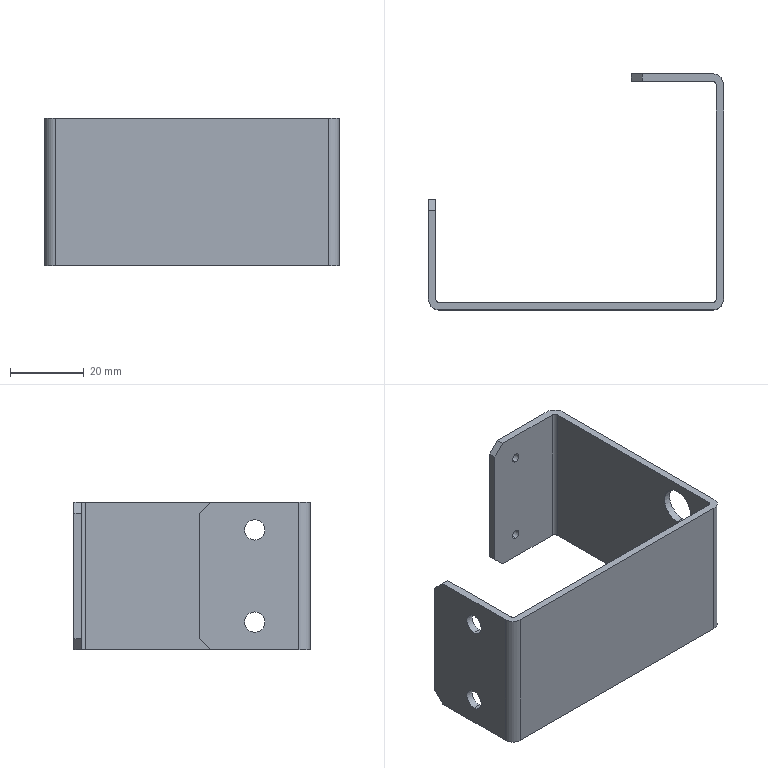Part | SolidWorks | features BaseBody 1 | 1 solid | 34 faces | box 80 x 64 x 40 mm | volume 14769 mm3 | cylinder 18 | plane 16 | commonest cylinder face diameters 2.5 x4 5.5 x4 10 x4 2 x3 6 x3
STEP:
#1=CARTESIAN_POINT('',(-80.,-49.,15.25));
#2=VERTEX_POINT('',#1);
#3=CARTESIAN_POINT('',(-80.,-49.,9.75));
#4=VERTEX_POINT('',#3);
#5=CARTESIAN_POINT('',(-80.,-49.,12.5));
#6=DIRECTION('',(1.,0.,0.));
#7=DIRECTION('',(0.,0.,-1.));
#8=AXIS2_PLACEMENT_3D('',#5,#6,#7);
#9=CIRCLE('',#8,2.75);
#10=EDGE_CURVE('',#2,#4,#9,.T.);
#11=ORIENTED_EDGE('',*,*,#10,.F.);
#12=CARTESIAN_POINT('',(-78.,-49.,15.25));
#13=VERTEX_POINT('',#12);
#14=CARTESIAN_POINT('',(0.,-49.,15.25));
#15=DIRECTION('',(1.,0.,0.));
#16=VECTOR('',#15,1000.);
#17=LINE('',#14,#16);
#18=EDGE_CURVE('',#2,#13,#17,.T.);
#19=ORIENTED_EDGE('',*,*,#18,.T.);
#20=CARTESIAN_POINT('',(-78.,-49.,9.75));
#21=VERTEX_POINT('',#20);
#22=CARTESIAN_POINT('',(-78.,-49.,12.5));
#23=DIRECTION('',(-1.,0.,0.));
#24=DIRECTION('',(0.,0.,1.));
#25=AXIS2_PLACEMENT_3D('',#22,#23,#24);
#26=CIRCLE('',#25,2.75);
#27=EDGE_CURVE('',#21,#13,#26,.T.);
#28=ORIENTED_EDGE('',*,*,#27,.F.);
#29=CARTESIAN_POINT('',(0.,-49.,9.75));
#30=DIRECTION('',(1.,0.,0.));
#31=VECTOR('',#30,1000.);
#32=LINE('',#29,#31);
#33=EDGE_CURVE('',#4,#21,#32,.T.);
#34=ORIENTED_EDGE('',*,*,#33,.F.);
#35=EDGE_LOOP('',(#11,#19,#28,#34));
#36=FACE_OUTER_BOUND('',#35,.T.);
#37=CARTESIAN_POINT('',(0.,-49.,12.5));
#38=DIRECTION('',(1.,0.,0.));
#39=DIRECTION('',(0.,0.,-1.));
#40=AXIS2_PLACEMENT_3D('',#37,#38,#39);
#41=CYLINDRICAL_SURFACE('',#40,2.75);
#42=ADVANCED_FACE('',(#36),#41,.F.);
#43=CARTESIAN_POINT('',(-2.,-49.,17.5));
#44=VERTEX_POINT('',#43);
#45=CARTESIAN_POINT('',(-2.,-49.,7.5));
#46=VERTEX_POINT('',#45);
#47=CARTESIAN_POINT('',(-2.,-49.,12.5));
#48=DIRECTION('',(1.,0.,0.));
#49=DIRECTION('',(0.,1.,0.));
#50=AXIS2_PLACEMENT_3D('',#47,#48,#49);
#51=CIRCLE('',#50,5.);
#52=EDGE_CURVE('',#44,#46,#51,.T.);
#53=ORIENTED_EDGE('',*,*,#52,.F.);
#54=CARTESIAN_POINT('',(0.,-49.,17.5));
#55=VERTEX_POINT('',#54);
#56=CARTESIAN_POINT('',(0.,-49.,17.5));
#57=DIRECTION('',(1.,0.,0.));
#58=VECTOR('',#57,1000.);
#59=LINE('',#56,#58);
#60=EDGE_CURVE('',#44,#55,#59,.T.);
#61=ORIENTED_EDGE('',*,*,#60,.T.);
#62=CARTESIAN_POINT('',(0.,-49.,7.5));
#63=VERTEX_POINT('',#62);
#64=CARTESIAN_POINT('',(0.,-49.,12.5));
#65=DIRECTION('',(1.,0.,0.));
#66=DIRECTION('',(0.,0.,-1.));
#67=AXIS2_PLACEMENT_3D('',#64,#65,#66);
#68=CIRCLE('',#67,5.);
#69=EDGE_CURVE('',#55,#63,#68,.T.);
#70=ORIENTED_EDGE('',*,*,#69,.T.);
#71=CARTESIAN_POINT('',(0.,-49.,7.5));
#72=DIRECTION('',(1.,0.,0.));
#73=VECTOR('',#72,1000.);
#74=LINE('',#71,#73);
#75=EDGE_CURVE('',#46,#63,#74,.T.);
#76=ORIENTED_EDGE('',*,*,#75,.F.);
#77=EDGE_LOOP('',(#53,#61,#70,#76));
#78=FACE_OUTER_BOUND('',#77,.T.);
#79=CARTESIAN_POINT('',(0.,-49.,12.5));
#80=DIRECTION('',(1.,0.,0.));
#81=DIRECTION('',(0.,0.,-1.));
#82=AXIS2_PLACEMENT_3D('',#79,#80,#81);
#83=CYLINDRICAL_SURFACE('',#82,5.);
#84=ADVANCED_FACE('',(#78),#83,.F.);
#85=CARTESIAN_POINT('',(-80.,-49.,-9.75));
#86=VERTEX_POINT('',#85);
#87=CARTESIAN_POINT('',(-80.,-49.,-15.25));
#88=VERTEX_POINT('',#87);
#89=CARTESIAN_POINT('',(-80.,-49.,-12.5));
#90=DIRECTION('',(1.,0.,0.));
#91=DIRECTION('',(0.,0.,-1.));
#92=AXIS2_PLACEMENT_3D('',#89,#90,#91);
#93=CIRCLE('',#92,2.75);
#94=EDGE_CURVE('',#86,#88,#93,.T.);
#95=ORIENTED_EDGE('',*,*,#94,.F.);
#96=CARTESIAN_POINT('',(-78.,-49.,-9.75));
#97=VERTEX_POINT('',#96);
#98=CARTESIAN_POINT('',(0.,-49.,-9.75));
#99=DIRECTION('',(1.,0.,0.));
#100=VECTOR('',#99,1000.);
#101=LINE('',#98,#100);
#102=EDGE_CURVE('',#86,#97,#101,.T.);
#103=ORIENTED_EDGE('',*,*,#102,.T.);
#104=CARTESIAN_POINT('',(-78.,-49.,-15.25));
#105=VERTEX_POINT('',#104);
#106=CARTESIAN_POINT('',(-78.,-49.,-12.5));
#107=DIRECTION('',(-1.,0.,0.));
#108=DIRECTION('',(0.,0.,1.));
#109=AXIS2_PLACEMENT_3D('',#106,#107,#108);
#110=CIRCLE('',#109,2.75);
#111=EDGE_CURVE('',#105,#97,#110,.T.);
#112=ORIENTED_EDGE('',*,*,#111,.F.);
#113=CARTESIAN_POINT('',(0.,-49.,-15.25));
#114=DIRECTION('',(1.,0.,0.));
#115=VECTOR('',#114,1000.);
#116=LINE('',#113,#115);
#117=EDGE_CURVE('',#88,#105,#116,.T.);
#118=ORIENTED_EDGE('',*,*,#117,.F.);
#119=EDGE_LOOP('',(#95,#103,#112,#118));
#120=FACE_OUTER_BOUND('',#119,.T.);
#121=CARTESIAN_POINT('',(0.,-49.,-12.5));
#122=DIRECTION('',(1.,0.,0.));
#123=DIRECTION('',(0.,0.,-1.));
#124=AXIS2_PLACEMENT_3D('',#121,#122,#123);
#125=CYLINDRICAL_SURFACE('',#124,2.75);
#126=ADVANCED_FACE('',(#120),#125,.F.);
#127=CARTESIAN_POINT('',(-2.,-49.,-7.5));
#128=VERTEX_POINT('',#127);
#129=CARTESIAN_POINT('',(-2.,-49.,-17.5));
#130=VERTEX_POINT('',#129);
#131=CARTESIAN_POINT('',(-2.,-49.,-12.5));
#132=DIRECTION('',(1.,0.,0.));
#133=DIRECTION('',(0.,1.,0.));
#134=AXIS2_PLACEMENT_3D('',#131,#132,#133);
#135=CIRCLE('',#134,5.);
#136=EDGE_CURVE('',#128,#130,#135,.T.);
#137=ORIENTED_EDGE('',*,*,#136,.F.);
#138=CARTESIAN_POINT('',(0.,-49.,-7.5));
#139=VERTEX_POINT('',#138);
#140=CARTESIAN_POINT('',(0.,-49.,-7.5));
#141=DIRECTION('',(1.,0.,0.));
#142=VECTOR('',#141,1000.);
#143=LINE('',#140,#142);
#144=EDGE_CURVE('',#128,#139,#143,.T.);
#145=ORIENTED_EDGE('',*,*,#144,.T.);
#146=CARTESIAN_POINT('',(0.,-49.,-17.5));
#147=VERTEX_POINT('',#146);
#148=CARTESIAN_POINT('',(0.,-49.,-12.5));
#149=DIRECTION('',(1.,0.,0.));
#150=DIRECTION('',(0.,0.,-1.));
#151=AXIS2_PLACEMENT_3D('',#148,#149,#150);
#152=CIRCLE('',#151,5.);
#153=EDGE_CURVE('',#139,#147,#152,.T.);
#154=ORIENTED_EDGE('',*,*,#153,.T.);
#155=CARTESIAN_POINT('',(0.,-49.,-17.5));
#156=DIRECTION('',(1.,0.,0.));
#157=VECTOR('',#156,1000.);
#158=LINE('',#155,#157);
#159=EDGE_CURVE('',#130,#147,#158,.T.);
#160=ORIENTED_EDGE('',*,*,#159,.F.);
#161=EDGE_LOOP('',(#137,#145,#154,#160));
#162=FACE_OUTER_BOUND('',#161,.T.);
#163=CARTESIAN_POINT('',(0.,-49.,-12.5));
#164=DIRECTION('',(1.,0.,0.));
#165=DIRECTION('',(0.,0.,-1.));
#166=AXIS2_PLACEMENT_3D('',#163,#164,#165);
#167=CYLINDRICAL_SURFACE('',#166,5.);
#168=ADVANCED_FACE('',(#162),#167,.F.);
#169=CARTESIAN_POINT('',(-17.,-2.,11.45));
#170=VERTEX_POINT('',#169);
#171=CARTESIAN_POINT('',(-17.,-2.,13.95));
#172=VERTEX_POINT('',#171);
#173=CARTESIAN_POINT('',(-17.,-2.,12.7));
#174=DIRECTION('',(0.,1.,0.));
#175=DIRECTION('',(0.,0.,1.));
#176=AXIS2_PLACEMENT_3D('',#173,#174,#175);
#177=CIRCLE('',#176,1.25);
#178=EDGE_CURVE('',#170,#172,#177,.T.);
#179=ORIENTED_EDGE('',*,*,#178,.F.);
#180=CARTESIAN_POINT('',(-17.,0.,11.45));
#181=VERTEX_POINT('',#180);
#182=CARTESIAN_POINT('',(-17.,0.,11.45));
#183=DIRECTION('',(0.,1.,0.));
#184=VECTOR('',#183,1000.);
#185=LINE('',#182,#184);
#186=EDGE_CURVE('',#170,#181,#185,.T.);
#187=ORIENTED_EDGE('',*,*,#186,.T.);
#188=CARTESIAN_POINT('',(-17.,0.,13.95));
#189=VERTEX_POINT('',#188);
#190=CARTESIAN_POINT('',(-17.,0.,12.7));
#191=DIRECTION('',(0.,1.,0.));
#192=DIRECTION('',(0.,0.,1.));
#193=AXIS2_PLACEMENT_3D('',#190,#191,#192);
#194=CIRCLE('',#193,1.25);
#195=EDGE_CURVE('',#181,#189,#194,.T.);
#196=ORIENTED_EDGE('',*,*,#195,.T.);
#197=CARTESIAN_POINT('',(-17.,0.,13.95));
#198=DIRECTION('',(0.,1.,0.));
#199=VECTOR('',#198,1000.);
#200=LINE('',#197,#199);
#201=EDGE_CURVE('',#172,#189,#200,.T.);
#202=ORIENTED_EDGE('',*,*,#201,.F.);
#203=EDGE_LOOP('',(#179,#187,#196,#202));
#204=FACE_OUTER_BOUND('',#203,.T.);
#205=CARTESIAN_POINT('',(-17.,0.,12.7));
#206=DIRECTION('',(0.,1.,0.));
#207=DIRECTION('',(0.,0.,1.));
#208=AXIS2_PLACEMENT_3D('',#205,#206,#207);
#209=CYLINDRICAL_SURFACE('',#208,1.25);
#210=ADVANCED_FACE('',(#204),#209,.F.);
#211=CARTESIAN_POINT('',(-17.,-2.,-13.95));
#212=VERTEX_POINT('',#211);
#213=CARTESIAN_POINT('',(-17.,-2.,-11.45));
#214=VERTEX_POINT('',#213);
#215=CARTESIAN_POINT('',(-17.,-2.,-12.7));
#216=DIRECTION('',(0.,1.,0.));
#217=DIRECTION('',(0.,0.,1.));
#218=AXIS2_PLACEMENT_3D('',#215,#216,#217);
#219=CIRCLE('',#218,1.25);
#220=EDGE_CURVE('',#212,#214,#219,.T.);
#221=ORIENTED_EDGE('',*,*,#220,.F.);
#222=CARTESIAN_POINT('',(-17.,0.,-13.95));
#223=VERTEX_POINT('',#222);
#224=CARTESIAN_POINT('',(-17.,0.,-13.95));
#225=DIRECTION('',(0.,1.,0.));
#226=VECTOR('',#225,1000.);
#227=LINE('',#224,#226);
#228=EDGE_CURVE('',#212,#223,#227,.T.);
#229=ORIENTED_EDGE('',*,*,#228,.T.);
#230=CARTESIAN_POINT('',(-17.,0.,-11.45));
#231=VERTEX_POINT('',#230);
#232=CARTESIAN_POINT('',(-17.,0.,-12.7));
#233=DIRECTION('',(0.,1.,0.));
#234=DIRECTION('',(0.,0.,1.));
#235=AXIS2_PLACEMENT_3D('',#232,#233,#234);
#236=CIRCLE('',#235,1.25);
#237=EDGE_CURVE('',#223,#231,#236,.T.);
#238=ORIENTED_EDGE('',*,*,#237,.T.);
#239=CARTESIAN_POINT('',(-17.,0.,-11.45));
#240=DIRECTION('',(0.,1.,0.));
#241=VECTOR('',#240,1000.);
#242=LINE('',#239,#241);
#243=EDGE_CURVE('',#214,#231,#242,.T.);
#244=ORIENTED_EDGE('',*,*,#243,.F.);
#245=EDGE_LOOP('',(#221,#229,#238,#244));
#246=FACE_OUTER_BOUND('',#245,.T.);
#247=CARTESIAN_POINT('',(-17.,0.,-12.7));
#248=DIRECTION('',(0.,1.,0.));
#249=DIRECTION('',(0.,0.,1.));
#250=AXIS2_PLACEMENT_3D('',#247,#248,#249);
#251=CYLINDRICAL_SURFACE('',#250,1.25);
#252=ADVANCED_FACE('',(#246),#251,.F.);
#253=CARTESIAN_POINT('',(-80.,-34.,-17.));
#254=VERTEX_POINT('',#253);
#255=CARTESIAN_POINT('',(-80.,-37.,-20.));
#256=VERTEX_POINT('',#255);
#257=CARTESIAN_POINT('',(-80.,-30.5,-13.5));
#258=DIRECTION('',(0.,-0.7071,-0.7071));
#259=VECTOR('',#258,1000.);
#260=LINE('',#257,#259);
#261=EDGE_CURVE('',#254,#256,#260,.T.);
#262=ORIENTED_EDGE('',*,*,#261,.F.);
#263=CARTESIAN_POINT('',(-78.,-34.,-17.));
#264=VERTEX_POINT('',#263);
#265=CARTESIAN_POINT('',(-80.,-34.,-17.));
#266=DIRECTION('',(-1.,0.,0.));
#267=VECTOR('',#266,1000.);
#268=LINE('',#265,#267);
#269=EDGE_CURVE('',#264,#254,#268,.T.);
#270=ORIENTED_EDGE('',*,*,#269,.F.);
#271=CARTESIAN_POINT('',(-78.,-37.,-20.));
#272=VERTEX_POINT('',#271);
#273=CARTESIAN_POINT('',(-78.,-37.,-20.));
#274=DIRECTION('',(0.,0.7071,0.7071));
#275=VECTOR('',#274,1000.);
#276=LINE('',#273,#275);
#277=EDGE_CURVE('',#272,#264,#276,.T.);
#278=ORIENTED_EDGE('',*,*,#277,.F.);
#279=CARTESIAN_POINT('',(-78.,-37.,-20.));
#280=DIRECTION('',(1.,0.,0.));
#281=VECTOR('',#280,1000.);
#282=LINE('',#279,#281);
#283=EDGE_CURVE('',#256,#272,#282,.T.);
#284=ORIENTED_EDGE('',*,*,#283,.F.);
#285=EDGE_LOOP('',(#262,#270,#278,#284));
#286=FACE_OUTER_BOUND('',#285,.T.);
#287=CARTESIAN_POINT('',(-77.,-37.,-20.));
#288=DIRECTION('',(0.,0.7071,-0.7071));
#289=DIRECTION('',(-1.,0.,0.));
#290=AXIS2_PLACEMENT_3D('',#287,#288,#289);
#291=PLANE('',#290);
#292=ADVANCED_FACE('',(#286),#291,.T.);
#293=CARTESIAN_POINT('',(-80.,-37.,20.));
#294=VERTEX_POINT('',#293);
#295=CARTESIAN_POINT('',(-80.,-34.,17.));
#296=VERTEX_POINT('',#295);
#297=CARTESIAN_POINT('',(-80.,-50.5,33.5));
#298=DIRECTION('',(0.,0.7071,-0.7071));
#299=VECTOR('',#298,1000.);
#300=LINE('',#297,#299);
#301=EDGE_CURVE('',#294,#296,#300,.T.);
#302=ORIENTED_EDGE('',*,*,#301,.F.);
#303=CARTESIAN_POINT('',(-78.,-37.,20.));
#304=VERTEX_POINT('',#303);
#305=CARTESIAN_POINT('',(-77.,-37.,20.));
#306=DIRECTION('',(-1.,0.,0.));
#307=VECTOR('',#306,1000.);
#308=LINE('',#305,#307);
#309=EDGE_CURVE('',#304,#294,#308,.T.);
#310=ORIENTED_EDGE('',*,*,#309,.F.);
#311=CARTESIAN_POINT('',(-78.,-34.,17.));
#312=VERTEX_POINT('',#311);
#313=CARTESIAN_POINT('',(-78.,-34.,17.));
#314=DIRECTION('',(0.,-0.7071,0.7071));
#315=VECTOR('',#314,1000.);
#316=LINE('',#313,#315);
#317=EDGE_CURVE('',#312,#304,#316,.T.);
#318=ORIENTED_EDGE('',*,*,#317,.F.);
#319=CARTESIAN_POINT('',(-80.,-34.,17.));
#320=DIRECTION('',(1.,0.,0.));
#321=VECTOR('',#320,1000.);
#322=LINE('',#319,#321);
#323=EDGE_CURVE('',#296,#312,#322,.T.);
#324=ORIENTED_EDGE('',*,*,#323,.F.);
#325=EDGE_LOOP('',(#302,#310,#318,#324));
#326=FACE_OUTER_BOUND('',#325,.T.);
#327=CARTESIAN_POINT('',(-80.,-34.,17.));
#328=DIRECTION('',(0.,-0.7071,-0.7071));
#329=DIRECTION('',(0.,-0.7071,0.7071));
#330=AXIS2_PLACEMENT_3D('',#327,#328,#329);
#331=PLANE('',#330);
#332=ADVANCED_FACE('',(#326),#331,.F.);
#333=CARTESIAN_POINT('',(-25.,-2.,-17.));
#334=VERTEX_POINT('',#333);
#335=CARTESIAN_POINT('',(-22.,-2.,-20.));
#336=VERTEX_POINT('',#335);
#337=CARTESIAN_POINT('',(-22.,-2.,-20.));
#338=DIRECTION('',(0.7071,0.,-0.7071));
#339=VECTOR('',#338,1000.);
#340=LINE('',#337,#339);
#341=EDGE_CURVE('',#334,#336,#340,.T.);
#342=ORIENTED_EDGE('',*,*,#341,.F.);
#343=CARTESIAN_POINT('',(-25.,0.,-17.));
#344=VERTEX_POINT('',#343);
#345=CARTESIAN_POINT('',(-25.,-2.,-17.));
#346=DIRECTION('',(0.,-1.,0.));
#347=VECTOR('',#346,1000.);
#348=LINE('',#345,#347);
#349=EDGE_CURVE('',#344,#334,#348,.T.);
#350=ORIENTED_EDGE('',*,*,#349,.F.);
#351=CARTESIAN_POINT('',(-22.,0.,-20.));
#352=VERTEX_POINT('',#351);
#353=CARTESIAN_POINT('',(-43.5,0.,1.5));
#354=DIRECTION('',(-0.7071,0.,0.7071));
#355=VECTOR('',#354,1000.);
#356=LINE('',#353,#355);
#357=EDGE_CURVE('',#352,#344,#356,.T.);
#358=ORIENTED_EDGE('',*,*,#357,.F.);
#359=CARTESIAN_POINT('',(-22.,-3.,-20.));
#360=DIRECTION('',(0.,1.,0.));
#361=VECTOR('',#360,1000.);
#362=LINE('',#359,#361);
#363=EDGE_CURVE('',#336,#352,#362,.T.);
#364=ORIENTED_EDGE('',*,*,#363,.F.);
#365=EDGE_LOOP('',(#342,#350,#358,#364));
#366=FACE_OUTER_BOUND('',#365,.T.);
#367=CARTESIAN_POINT('',(-22.,-3.,-20.));
#368=DIRECTION('',(0.7071,0.,0.7071));
#369=DIRECTION('',(0.,-1.,0.));
#370=AXIS2_PLACEMENT_3D('',#367,#368,#369);
#371=PLANE('',#370);
#372=ADVANCED_FACE('',(#366),#371,.F.);
#373=CARTESIAN_POINT('',(-22.,-2.,20.));
#374=VERTEX_POINT('',#373);
#375=CARTESIAN_POINT('',(-25.,-2.,17.));
#376=VERTEX_POINT('',#375);
#377=CARTESIAN_POINT('',(-25.,-2.,17.));
#378=DIRECTION('',(-0.7071,0.,-0.7071));
#379=VECTOR('',#378,1000.);
#380=LINE('',#377,#379);
#381=EDGE_CURVE('',#374,#376,#380,.T.);
#382=ORIENTED_EDGE('',*,*,#381,.F.);
#383=CARTESIAN_POINT('',(-22.,0.,20.));
#384=VERTEX_POINT('',#383);
#385=CARTESIAN_POINT('',(-22.,-61.,20.));
#386=DIRECTION('',(0.,-1.,0.));
#387=VECTOR('',#386,1000.);
#388=LINE('',#385,#387);
#389=EDGE_CURVE('',#384,#374,#388,.T.);
#390=ORIENTED_EDGE('',*,*,#389,.F.);
#391=CARTESIAN_POINT('',(-25.,0.,17.));
#392=VERTEX_POINT('',#391);
#393=CARTESIAN_POINT('',(-23.5,0.,18.5));
#394=DIRECTION('',(0.7071,0.,0.7071));
#395=VECTOR('',#394,1000.);
#396=LINE('',#393,#395);
#397=EDGE_CURVE('',#392,#384,#396,.T.);
#398=ORIENTED_EDGE('',*,*,#397,.F.);
#399=CARTESIAN_POINT('',(-25.,-2.,17.));
#400=DIRECTION('',(0.,1.,0.));
#401=VECTOR('',#400,1000.);
#402=LINE('',#399,#401);
#403=EDGE_CURVE('',#376,#392,#402,.T.);
#404=ORIENTED_EDGE('',*,*,#403,.F.);
#405=EDGE_LOOP('',(#382,#390,#398,#404));
#406=FACE_OUTER_BOUND('',#405,.T.);
#407=CARTESIAN_POINT('',(-25.,-2.,17.));
#408=DIRECTION('',(0.7071,0.,-0.7071));
#409=DIRECTION('',(0.,-1.,0.));
#410=AXIS2_PLACEMENT_3D('',#407,#408,#409);
#411=PLANE('',#410);
#412=ADVANCED_FACE('',(#406),#411,.F.);
#413=CARTESIAN_POINT('',(-77.,-62.,-20.));
#414=VERTEX_POINT('',#413);
#415=CARTESIAN_POINT('',(-78.,-61.,-20.));
#416=VERTEX_POINT('',#415);
#417=CARTESIAN_POINT('',(-77.,-61.,-20.));
#418=DIRECTION('',(0.,0.,-1.));
#419=DIRECTION('',(1.,0.,0.));
#420=AXIS2_PLACEMENT_3D('',#417,#418,#419);
#421=CIRCLE('',#420,1.);
#422=EDGE_CURVE('',#414,#416,#421,.T.);
#423=ORIENTED_EDGE('',*,*,#422,.T.);
#424=CARTESIAN_POINT('',(-78.,-61.,20.));
#425=VERTEX_POINT('',#424);
#426=CARTESIAN_POINT('',(-78.,-61.,20.));
#427=DIRECTION('',(0.,0.,-1.));
#428=VECTOR('',#427,1000.);
#429=LINE('',#426,#428);
#430=EDGE_CURVE('',#425,#416,#429,.T.);
#431=ORIENTED_EDGE('',*,*,#430,.F.);
#432=CARTESIAN_POINT('',(-77.,-62.,20.));
#433=VERTEX_POINT('',#432);
#434=CARTESIAN_POINT('',(-77.,-61.,20.));
#435=DIRECTION('',(0.,0.,-1.));
#436=DIRECTION('',(1.,0.,0.));
#437=AXIS2_PLACEMENT_3D('',#434,#435,#436);
#438=CIRCLE('',#437,1.);
#439=EDGE_CURVE('',#433,#425,#438,.T.);
#440=ORIENTED_EDGE('',*,*,#439,.F.);
#441=CARTESIAN_POINT('',(-77.,-62.,20.));
#442=DIRECTION('',(0.,0.,-1.));
#443=VECTOR('',#442,1000.);
#444=LINE('',#441,#443);
#445=EDGE_CURVE('',#433,#414,#444,.T.);
#446=ORIENTED_EDGE('',*,*,#445,.T.);
#447=EDGE_LOOP('',(#423,#431,#440,#446));
#448=FACE_OUTER_BOUND('',#447,.T.);
#449=CARTESIAN_POINT('',(-77.,-61.,20.));
#450=DIRECTION('',(0.,0.,-1.));
#451=DIRECTION('',(-1.,0.,0.));
#452=AXIS2_PLACEMENT_3D('',#449,#450,#451);
#453=CYLINDRICAL_SURFACE('',#452,1.);
#454=ADVANCED_FACE('',(#448),#453,.F.);
#455=CARTESIAN_POINT('',(-3.,-62.,-20.));
#456=VERTEX_POINT('',#455);
#457=CARTESIAN_POINT('',(0.,-62.,-20.));
#458=DIRECTION('',(-1.,0.,0.));
#459=VECTOR('',#458,1000.);
#460=LINE('',#457,#459);
#461=EDGE_CURVE('',#456,#414,#460,.T.);
#462=ORIENTED_EDGE('',*,*,#461,.T.);
#463=ORIENTED_EDGE('',*,*,#445,.F.);
#464=CARTESIAN_POINT('',(-3.,-62.,20.));
#465=VERTEX_POINT('',#464);
#466=CARTESIAN_POINT('',(0.,-62.,20.));
#467=DIRECTION('',(-1.,0.,0.));
#468=VECTOR('',#467,1000.);
#469=LINE('',#466,#468);
#470=EDGE_CURVE('',#465,#433,#469,.T.);
#471=ORIENTED_EDGE('',*,*,#470,.F.);
#472=CARTESIAN_POINT('',(-3.,-62.,20.));
#473=DIRECTION('',(0.,0.,-1.));
#474=VECTOR('',#473,1000.);
#475=LINE('',#472,#474);
#476=EDGE_CURVE('',#465,#456,#475,.T.);
#477=ORIENTED_EDGE('',*,*,#476,.T.);
#478=EDGE_LOOP('',(#462,#463,#471,#477));
#479=FACE_OUTER_BOUND('',#478,.T.);
#480=CARTESIAN_POINT('',(0.,-62.,20.));
#481=DIRECTION('',(0.,-1.,0.));
#482=DIRECTION('',(0.,0.,-1.));
#483=AXIS2_PLACEMENT_3D('',#480,#481,#482);
#484=PLANE('',#483);
#485=ADVANCED_FACE('',(#479),#484,.F.);
#486=CARTESIAN_POINT('',(-2.,-61.,-20.));
#487=VERTEX_POINT('',#486);
#488=CARTESIAN_POINT('',(-3.,-61.,-20.));
#489=DIRECTION('',(0.,0.,-1.));
#490=DIRECTION('',(1.,0.,0.));
#491=AXIS2_PLACEMENT_3D('',#488,#489,#490);
#492=CIRCLE('',#491,1.);
#493=EDGE_CURVE('',#487,#456,#492,.T.);
#494=ORIENTED_EDGE('',*,*,#493,.T.);
#495=ORIENTED_EDGE('',*,*,#476,.F.);
#496=CARTESIAN_POINT('',(-2.,-61.,20.));
#497=VERTEX_POINT('',#496);
#498=CARTESIAN_POINT('',(-3.,-61.,20.));
#499=DIRECTION('',(0.,0.,-1.));
#500=DIRECTION('',(1.,0.,0.));
#501=AXIS2_PLACEMENT_3D('',#498,#499,#500);
#502=CIRCLE('',#501,1.);
#503=EDGE_CURVE('',#497,#465,#502,.T.);
#504=ORIENTED_EDGE('',*,*,#503,.F.);
#505=CARTESIAN_POINT('',(-2.,-61.,20.));
#506=DIRECTION('',(0.,0.,-1.));
#507=VECTOR('',#506,1000.);
#508=LINE('',#505,#507);
#509=EDGE_CURVE('',#497,#487,#508,.T.);
#510=ORIENTED_EDGE('',*,*,#509,.T.);
#511=EDGE_LOOP('',(#494,#495,#504,#510));
#512=FACE_OUTER_BOUND('',#511,.T.);
#513=CARTESIAN_POINT('',(-3.,-61.,20.));
#514=DIRECTION('',(0.,0.,-1.));
#515=DIRECTION('',(-1.,0.,0.));
#516=AXIS2_PLACEMENT_3D('',#513,#514,#515);
#517=CYLINDRICAL_SURFACE('',#516,1.);
#518=ADVANCED_FACE('',(#512),#517,.F.);
#519=CARTESIAN_POINT('',(-2.,-49.,-12.5));
#520=DIRECTION('',(1.,0.,0.));
#521=DIRECTION('',(0.,1.,0.));
#522=AXIS2_PLACEMENT_3D('',#519,#520,#521);
#523=CIRCLE('',#522,5.);
#524=EDGE_CURVE('',#130,#128,#523,.T.);
#525=ORIENTED_EDGE('',*,*,#524,.T.);
#526=ORIENTED_EDGE('',*,*,#136,.T.);
#527=EDGE_LOOP('',(#525,#526));
#528=FACE_BOUND('',#527,.T.);
#529=CARTESIAN_POINT('',(-2.,-49.,12.5));
#530=DIRECTION('',(1.,0.,0.));
#531=DIRECTION('',(0.,1.,0.));
#532=AXIS2_PLACEMENT_3D('',#529,#530,#531);
#533=CIRCLE('',#532,5.);
#534=EDGE_CURVE('',#46,#44,#533,.T.);
#535=ORIENTED_EDGE('',*,*,#534,.T.);
#536=ORIENTED_EDGE('',*,*,#52,.T.);
#537=EDGE_LOOP('',(#535,#536));
#538=FACE_BOUND('',#537,.T.);
#539=CARTESIAN_POINT('',(-2.,-3.,-20.));
#540=VERTEX_POINT('',#539);
#541=CARTESIAN_POINT('',(-2.,0.,-20.));
#542=DIRECTION('',(0.,-1.,0.));
#543=VECTOR('',#542,1000.);
#544=LINE('',#541,#543);
#545=EDGE_CURVE('',#540,#487,#544,.T.);
#546=ORIENTED_EDGE('',*,*,#545,.T.);
#547=ORIENTED_EDGE('',*,*,#509,.F.);
#548=CARTESIAN_POINT('',(-2.,-3.,20.));
#549=VERTEX_POINT('',#548);
#550=CARTESIAN_POINT('',(-2.,0.,20.));
#551=DIRECTION('',(0.,-1.,0.));
#552=VECTOR('',#551,1000.);
#553=LINE('',#550,#552);
#554=EDGE_CURVE('',#549,#497,#553,.T.);
#555=ORIENTED_EDGE('',*,*,#554,.F.);
#556=CARTESIAN_POINT('',(-2.,-3.,20.));
#557=DIRECTION('',(0.,0.,-1.));
#558=VECTOR('',#557,1000.);
#559=LINE('',#556,#558);
#560=EDGE_CURVE('',#549,#540,#559,.T.);
#561=ORIENTED_EDGE('',*,*,#560,.T.);
#562=EDGE_LOOP('',(#546,#547,#555,#561));
#563=FACE_OUTER_BOUND('',#562,.T.);
#564=CARTESIAN_POINT('',(-2.,0.,20.));
#565=DIRECTION('',(1.,0.,0.));
#566=DIRECTION('',(0.,1.,0.));
#567=AXIS2_PLACEMENT_3D('',#564,#565,#566);
#568=PLANE('',#567);
#569=ADVANCED_FACE('',(#528,#538,#563),#568,.F.);
#570=CARTESIAN_POINT('',(-3.,-2.,-20.));
#571=VERTEX_POINT('',#570);
#572=CARTESIAN_POINT('',(-3.,-3.,-20.));
#573=DIRECTION('',(0.,0.,-1.));
#574=DIRECTION('',(1.,0.,0.));
#575=AXIS2_PLACEMENT_3D('',#572,#573,#574);
#576=CIRCLE('',#575,1.);
#577=EDGE_CURVE('',#571,#540,#576,.T.);
#578=ORIENTED_EDGE('',*,*,#577,.T.);
#579=ORIENTED_EDGE('',*,*,#560,.F.);
#580=CARTESIAN_POINT('',(-3.,-2.,20.));
#581=VERTEX_POINT('',#580);
#582=CARTESIAN_POINT('',(-3.,-3.,20.));
#583=DIRECTION('',(0.,0.,-1.));
#584=DIRECTION('',(1.,0.,0.));
#585=AXIS2_PLACEMENT_3D('',#582,#583,#584);
#586=CIRCLE('',#585,1.);
#587=EDGE_CURVE('',#581,#549,#586,.T.);
#588=ORIENTED_EDGE('',*,*,#587,.F.);
#589=CARTESIAN_POINT('',(-3.,-2.,20.));
#590=DIRECTION('',(0.,0.,-1.));
#591=VECTOR('',#590,1000.);
#592=LINE('',#589,#591);
#593=EDGE_CURVE('',#581,#571,#592,.T.);
#594=ORIENTED_EDGE('',*,*,#593,.T.);
#595=EDGE_LOOP('',(#578,#579,#588,#594));
#596=FACE_OUTER_BOUND('',#595,.T.);
#597=CARTESIAN_POINT('',(-3.,-3.,20.));
#598=DIRECTION('',(0.,0.,-1.));
#599=DIRECTION('',(-1.,0.,0.));
#600=AXIS2_PLACEMENT_3D('',#597,#598,#599);
#601=CYLINDRICAL_SURFACE('',#600,1.);
#602=ADVANCED_FACE('',(#596),#601,.F.);
#603=CARTESIAN_POINT('',(-17.,-2.,-12.7));
#604=DIRECTION('',(0.,1.,0.));
#605=DIRECTION('',(0.,0.,1.));
#606=AXIS2_PLACEMENT_3D('',#603,#604,#605);
#607=CIRCLE('',#606,1.25);
#608=EDGE_CURVE('',#214,#212,#607,.T.);
#609=ORIENTED_EDGE('',*,*,#608,.T.);
#610=ORIENTED_EDGE('',*,*,#220,.T.);
#611=EDGE_LOOP('',(#609,#610));
#612=FACE_BOUND('',#611,.T.);
#613=CARTESIAN_POINT('',(-17.,-2.,12.7));
#614=DIRECTION('',(0.,1.,0.));
#615=DIRECTION('',(0.,0.,1.));
#616=AXIS2_PLACEMENT_3D('',#613,#614,#615);
#617=CIRCLE('',#616,1.25);
#618=EDGE_CURVE('',#172,#170,#617,.T.);
#619=ORIENTED_EDGE('',*,*,#618,.T.);
#620=ORIENTED_EDGE('',*,*,#178,.T.);
#621=EDGE_LOOP('',(#619,#620));
#622=FACE_BOUND('',#621,.T.);
#623=CARTESIAN_POINT('',(-25.,-2.,20.));
#624=DIRECTION('',(1.,0.,0.));
#625=VECTOR('',#624,1000.);
#626=LINE('',#623,#625);
#627=EDGE_CURVE('',#374,#581,#626,.T.);
#628=ORIENTED_EDGE('',*,*,#627,.F.);
#629=ORIENTED_EDGE('',*,*,#381,.T.);
#630=CARTESIAN_POINT('',(-25.,-2.,20.));
#631=DIRECTION('',(0.,0.,-1.));
#632=VECTOR('',#631,1000.);
#633=LINE('',#630,#632);
#634=EDGE_CURVE('',#376,#334,#633,.T.);
#635=ORIENTED_EDGE('',*,*,#634,.T.);
#636=ORIENTED_EDGE('',*,*,#341,.T.);
#637=CARTESIAN_POINT('',(-25.,-2.,-20.));
#638=DIRECTION('',(1.,0.,0.));
#639=VECTOR('',#638,1000.);
#640=LINE('',#637,#639);
#641=EDGE_CURVE('',#336,#571,#640,.T.);
#642=ORIENTED_EDGE('',*,*,#641,.T.);
#643=ORIENTED_EDGE('',*,*,#593,.F.);
#644=EDGE_LOOP('',(#628,#629,#635,#636,#642,#643));
#645=FACE_OUTER_BOUND('',#644,.T.);
#646=CARTESIAN_POINT('',(-25.,-2.,20.));
#647=DIRECTION('',(0.,1.,0.));
#648=DIRECTION('',(1.,0.,0.));
#649=AXIS2_PLACEMENT_3D('',#646,#647,#648);
#650=PLANE('',#649);
#651=ADVANCED_FACE('',(#612,#622,#645),#650,.F.);
#652=ORIENTED_EDGE('',*,*,#634,.F.);
#653=ORIENTED_EDGE('',*,*,#403,.T.);
#654=CARTESIAN_POINT('',(-25.,0.,20.));
#655=DIRECTION('',(0.,0.,-1.));
#656=VECTOR('',#655,1000.);
#657=LINE('',#654,#656);
#658=EDGE_CURVE('',#392,#344,#657,.T.);
#659=ORIENTED_EDGE('',*,*,#658,.T.);
#660=ORIENTED_EDGE('',*,*,#349,.T.);
#661=EDGE_LOOP('',(#652,#653,#659,#660));
#662=FACE_OUTER_BOUND('',#661,.T.);
#663=CARTESIAN_POINT('',(-25.,-2.,20.));
#664=DIRECTION('',(-1.,0.,0.));
#665=DIRECTION('',(0.,0.,1.));
#666=AXIS2_PLACEMENT_3D('',#663,#664,#665);
#667=PLANE('',#666);
#668=ADVANCED_FACE('',(#662),#667,.T.);
#669=CARTESIAN_POINT('',(-17.,0.,-12.7));
#670=DIRECTION('',(0.,1.,0.));
#671=DIRECTION('',(0.,0.,1.));
#672=AXIS2_PLACEMENT_3D('',#669,#670,#671);
#673=CIRCLE('',#672,1.25);
#674=EDGE_CURVE('',#231,#223,#673,.T.);
#675=ORIENTED_EDGE('',*,*,#674,.F.);
#676=ORIENTED_EDGE('',*,*,#237,.F.);
#677=EDGE_LOOP('',(#675,#676));
#678=FACE_BOUND('',#677,.T.);
#679=CARTESIAN_POINT('',(-17.,0.,12.7));
#680=DIRECTION('',(0.,1.,0.));
#681=DIRECTION('',(0.,0.,1.));
#682=AXIS2_PLACEMENT_3D('',#679,#680,#681);
#683=CIRCLE('',#682,1.25);
#684=EDGE_CURVE('',#189,#181,#683,.T.);
#685=ORIENTED_EDGE('',*,*,#684,.F.);
#686=ORIENTED_EDGE('',*,*,#195,.F.);
#687=EDGE_LOOP('',(#685,#686));
#688=FACE_BOUND('',#687,.T.);
#689=ORIENTED_EDGE('',*,*,#658,.F.);
#690=ORIENTED_EDGE('',*,*,#397,.T.);
#691=CARTESIAN_POINT('',(-3.,0.,20.));
#692=VERTEX_POINT('',#691);
#693=CARTESIAN_POINT('',(-25.,0.,20.));
#694=DIRECTION('',(1.,0.,0.));
#695=VECTOR('',#694,1000.);
#696=LINE('',#693,#695);
#697=EDGE_CURVE('',#384,#692,#696,.T.);
#698=ORIENTED_EDGE('',*,*,#697,.T.);
#699=CARTESIAN_POINT('',(-3.,0.,-20.));
#700=VERTEX_POINT('',#699);
#701=CARTESIAN_POINT('',(-3.,0.,20.));
#702=DIRECTION('',(0.,0.,-1.));
#703=VECTOR('',#702,1000.);
#704=LINE('',#701,#703);
#705=EDGE_CURVE('',#692,#700,#704,.T.);
#706=ORIENTED_EDGE('',*,*,#705,.T.);
#707=CARTESIAN_POINT('',(-25.,0.,-20.));
#708=DIRECTION('',(1.,0.,0.));
#709=VECTOR('',#708,1000.);
#710=LINE('',#707,#709);
#711=EDGE_CURVE('',#352,#700,#710,.T.);
#712=ORIENTED_EDGE('',*,*,#711,.F.);
#713=ORIENTED_EDGE('',*,*,#357,.T.);
#714=EDGE_LOOP('',(#689,#690,#698,#706,#712,#713));
#715=FACE_OUTER_BOUND('',#714,.T.);
#716=CARTESIAN_POINT('',(-25.,0.,20.));
#717=DIRECTION('',(0.,1.,0.));
#718=DIRECTION('',(1.,0.,0.));
#719=AXIS2_PLACEMENT_3D('',#716,#717,#718);
#720=PLANE('',#719);
#721=ADVANCED_FACE('',(#678,#688,#715),#720,.T.);
#722=CARTESIAN_POINT('',(0.,-3.,-20.));
#723=VERTEX_POINT('',#722);
#724=CARTESIAN_POINT('',(-3.,-3.,-20.));
#725=DIRECTION('',(0.,0.,-1.));
#726=DIRECTION('',(1.,0.,0.));
#727=AXIS2_PLACEMENT_3D('',#724,#725,#726);
#728=CIRCLE('',#727,3.);
#729=EDGE_CURVE('',#700,#723,#728,.T.);
#730=ORIENTED_EDGE('',*,*,#729,.F.);
#731=ORIENTED_EDGE('',*,*,#705,.F.);
#732=CARTESIAN_POINT('',(0.,-3.,20.));
#733=VERTEX_POINT('',#732);
#734=CARTESIAN_POINT('',(-3.,-3.,20.));
#735=DIRECTION('',(0.,0.,-1.));
#736=DIRECTION('',(1.,0.,0.));
#737=AXIS2_PLACEMENT_3D('',#734,#735,#736);
#738=CIRCLE('',#737,3.);
#739=EDGE_CURVE('',#692,#733,#738,.T.);
#740=ORIENTED_EDGE('',*,*,#739,.T.);
#741=CARTESIAN_POINT('',(0.,-3.,20.));
#742=DIRECTION('',(0.,0.,-1.));
#743=VECTOR('',#742,1000.);
#744=LINE('',#741,#743);
#745=EDGE_CURVE('',#733,#723,#744,.T.);
#746=ORIENTED_EDGE('',*,*,#745,.T.);
#747=EDGE_LOOP('',(#730,#731,#740,#746));
#748=FACE_OUTER_BOUND('',#747,.T.);
#749=CARTESIAN_POINT('',(-3.,-3.,20.));
#750=DIRECTION('',(0.,0.,-1.));
#751=DIRECTION('',(-1.,0.,0.));
#752=AXIS2_PLACEMENT_3D('',#749,#750,#751);
#753=CYLINDRICAL_SURFACE('',#752,3.);
#754=ADVANCED_FACE('',(#748),#753,.T.);
#755=CARTESIAN_POINT('',(0.,-49.,-12.5));
#756=DIRECTION('',(1.,0.,0.));
#757=DIRECTION('',(0.,0.,-1.));
#758=AXIS2_PLACEMENT_3D('',#755,#756,#757);
#759=CIRCLE('',#758,5.);
#760=EDGE_CURVE('',#147,#139,#759,.T.);
#761=ORIENTED_EDGE('',*,*,#760,.F.);
#762=ORIENTED_EDGE('',*,*,#153,.F.);
#763=EDGE_LOOP('',(#761,#762));
#764=FACE_BOUND('',#763,.T.);
#765=CARTESIAN_POINT('',(0.,-49.,12.5));
#766=DIRECTION('',(1.,0.,0.));
#767=DIRECTION('',(0.,0.,-1.));
#768=AXIS2_PLACEMENT_3D('',#765,#766,#767);
#769=CIRCLE('',#768,5.);
#770=EDGE_CURVE('',#63,#55,#769,.T.);
#771=ORIENTED_EDGE('',*,*,#770,.F.);
#772=ORIENTED_EDGE('',*,*,#69,.F.);
#773=EDGE_LOOP('',(#771,#772));
#774=FACE_BOUND('',#773,.T.);
#775=CARTESIAN_POINT('',(0.,-61.,-20.));
#776=VERTEX_POINT('',#775);
#777=CARTESIAN_POINT('',(0.,0.,-20.));
#778=DIRECTION('',(0.,-1.,0.));
#779=VECTOR('',#778,1000.);
#780=LINE('',#777,#779);
#781=EDGE_CURVE('',#723,#776,#780,.T.);
#782=ORIENTED_EDGE('',*,*,#781,.F.);
#783=ORIENTED_EDGE('',*,*,#745,.F.);
#784=CARTESIAN_POINT('',(0.,-61.,20.));
#785=VERTEX_POINT('',#784);
#786=CARTESIAN_POINT('',(0.,0.,20.));
#787=DIRECTION('',(0.,-1.,0.));
#788=VECTOR('',#787,1000.);
#789=LINE('',#786,#788);
#790=EDGE_CURVE('',#733,#785,#789,.T.);
#791=ORIENTED_EDGE('',*,*,#790,.T.);
#792=CARTESIAN_POINT('',(0.,-61.,20.));
#793=DIRECTION('',(0.,0.,-1.));
#794=VECTOR('',#793,1000.);
#795=LINE('',#792,#794);
#796=EDGE_CURVE('',#785,#776,#795,.T.);
#797=ORIENTED_EDGE('',*,*,#796,.T.);
#798=EDGE_LOOP('',(#782,#783,#791,#797));
#799=FACE_OUTER_BOUND('',#798,.T.);
#800=CARTESIAN_POINT('',(0.,0.,20.));
#801=DIRECTION('',(1.,0.,0.));
#802=DIRECTION('',(0.,1.,0.));
#803=AXIS2_PLACEMENT_3D('',#800,#801,#802);
#804=PLANE('',#803);
#805=ADVANCED_FACE('',(#764,#774,#799),#804,.T.);
#806=CARTESIAN_POINT('',(-3.,-64.,-20.));
#807=VERTEX_POINT('',#806);
#808=CARTESIAN_POINT('',(-3.,-61.,-20.));
#809=DIRECTION('',(0.,0.,-1.));
#810=DIRECTION('',(1.,0.,0.));
#811=AXIS2_PLACEMENT_3D('',#808,#809,#810);
#812=CIRCLE('',#811,3.);
#813=EDGE_CURVE('',#776,#807,#812,.T.);
#814=ORIENTED_EDGE('',*,*,#813,.F.);
#815=ORIENTED_EDGE('',*,*,#796,.F.);
#816=CARTESIAN_POINT('',(-3.,-64.,20.));
#817=VERTEX_POINT('',#816);
#818=CARTESIAN_POINT('',(-3.,-61.,20.));
#819=DIRECTION('',(0.,0.,-1.));
#820=DIRECTION('',(1.,0.,0.));
#821=AXIS2_PLACEMENT_3D('',#818,#819,#820);
#822=CIRCLE('',#821,3.);
#823=EDGE_CURVE('',#785,#817,#822,.T.);
#824=ORIENTED_EDGE('',*,*,#823,.T.);
#825=CARTESIAN_POINT('',(-3.,-64.,20.));
#826=DIRECTION('',(0.,0.,-1.));
#827=VECTOR('',#826,1000.);
#828=LINE('',#825,#827);
#829=EDGE_CURVE('',#817,#807,#828,.T.);
#830=ORIENTED_EDGE('',*,*,#829,.T.);
#831=EDGE_LOOP('',(#814,#815,#824,#830));
#832=FACE_OUTER_BOUND('',#831,.T.);
#833=CARTESIAN_POINT('',(-3.,-61.,20.));
#834=DIRECTION('',(0.,0.,-1.));
#835=DIRECTION('',(-1.,0.,0.));
#836=AXIS2_PLACEMENT_3D('',#833,#834,#835);
#837=CYLINDRICAL_SURFACE('',#836,3.);
#838=ADVANCED_FACE('',(#832),#837,.T.);
#839=CARTESIAN_POINT('',(-77.,-64.,-20.));
#840=VERTEX_POINT('',#839);
#841=CARTESIAN_POINT('',(0.,-64.,-20.));
#842=DIRECTION('',(-1.,0.,0.));
#843=VECTOR('',#842,1000.);
#844=LINE('',#841,#843);
#845=EDGE_CURVE('',#807,#840,#844,.T.);
#846=ORIENTED_EDGE('',*,*,#845,.F.);
#847=ORIENTED_EDGE('',*,*,#829,.F.);
#848=CARTESIAN_POINT('',(-77.,-64.,20.));
#849=VERTEX_POINT('',#848);
#850=CARTESIAN_POINT('',(0.,-64.,20.));
#851=DIRECTION('',(-1.,0.,0.));
#852=VECTOR('',#851,1000.);
#853=LINE('',#850,#852);
#854=EDGE_CURVE('',#817,#849,#853,.T.);
#855=ORIENTED_EDGE('',*,*,#854,.T.);
#856=CARTESIAN_POINT('',(-77.,-64.,20.));
#857=DIRECTION('',(0.,0.,-1.));
#858=VECTOR('',#857,1000.);
#859=LINE('',#856,#858);
#860=EDGE_CURVE('',#849,#840,#859,.T.);
#861=ORIENTED_EDGE('',*,*,#860,.T.);
#862=EDGE_LOOP('',(#846,#847,#855,#861));
#863=FACE_OUTER_BOUND('',#862,.T.);
#864=CARTESIAN_POINT('',(0.,-64.,20.));
#865=DIRECTION('',(0.,-1.,0.));
#866=DIRECTION('',(0.,0.,-1.));
#867=AXIS2_PLACEMENT_3D('',#864,#865,#866);
#868=PLANE('',#867);
#869=ADVANCED_FACE('',(#863),#868,.T.);
#870=CARTESIAN_POINT('',(-80.,-61.,-20.));
#871=VERTEX_POINT('',#870);
#872=CARTESIAN_POINT('',(-77.,-61.,-20.));
#873=DIRECTION('',(0.,0.,-1.));
#874=DIRECTION('',(1.,0.,0.));
#875=AXIS2_PLACEMENT_3D('',#872,#873,#874);
#876=CIRCLE('',#875,3.);
#877=EDGE_CURVE('',#840,#871,#876,.T.);
#878=ORIENTED_EDGE('',*,*,#877,.F.);
#879=ORIENTED_EDGE('',*,*,#860,.F.);
#880=CARTESIAN_POINT('',(-80.,-61.,20.));
#881=VERTEX_POINT('',#880);
#882=CARTESIAN_POINT('',(-77.,-61.,20.));
#883=DIRECTION('',(0.,0.,-1.));
#884=DIRECTION('',(1.,0.,0.));
#885=AXIS2_PLACEMENT_3D('',#882,#883,#884);
#886=CIRCLE('',#885,3.);
#887=EDGE_CURVE('',#849,#881,#886,.T.);
#888=ORIENTED_EDGE('',*,*,#887,.T.);
#889=CARTESIAN_POINT('',(-80.,-61.,20.));
#890=DIRECTION('',(0.,0.,-1.));
#891=VECTOR('',#890,1000.);
#892=LINE('',#889,#891);
#893=EDGE_CURVE('',#881,#871,#892,.T.);
#894=ORIENTED_EDGE('',*,*,#893,.T.);
#895=EDGE_LOOP('',(#878,#879,#888,#894));
#896=FACE_OUTER_BOUND('',#895,.T.);
#897=CARTESIAN_POINT('',(-77.,-61.,20.));
#898=DIRECTION('',(0.,0.,-1.));
#899=DIRECTION('',(-1.,0.,0.));
#900=AXIS2_PLACEMENT_3D('',#897,#898,#899);
#901=CYLINDRICAL_SURFACE('',#900,3.);
#902=ADVANCED_FACE('',(#896),#901,.T.);
#903=CARTESIAN_POINT('',(-80.,-49.,-12.5));
#904=DIRECTION('',(1.,0.,0.));
#905=DIRECTION('',(0.,0.,-1.));
#906=AXIS2_PLACEMENT_3D('',#903,#904,#905);
#907=CIRCLE('',#906,2.75);
#908=EDGE_CURVE('',#88,#86,#907,.T.);
#909=ORIENTED_EDGE('',*,*,#908,.T.);
#910=ORIENTED_EDGE('',*,*,#94,.T.);
#911=EDGE_LOOP('',(#909,#910));
#912=FACE_BOUND('',#911,.T.);
#913=CARTESIAN_POINT('',(-80.,-49.,12.5));
#914=DIRECTION('',(1.,0.,0.));
#915=DIRECTION('',(0.,0.,-1.));
#916=AXIS2_PLACEMENT_3D('',#913,#914,#915);
#917=CIRCLE('',#916,2.75);
#918=EDGE_CURVE('',#4,#2,#917,.T.);
#919=ORIENTED_EDGE('',*,*,#918,.T.);
#920=ORIENTED_EDGE('',*,*,#10,.T.);
#921=EDGE_LOOP('',(#919,#920));
#922=FACE_BOUND('',#921,.T.);
#923=CARTESIAN_POINT('',(-80.,-64.,20.));
#924=DIRECTION('',(0.,1.,0.));
#925=VECTOR('',#924,1000.);
#926=LINE('',#923,#925);
#927=EDGE_CURVE('',#881,#294,#926,.T.);
#928=ORIENTED_EDGE('',*,*,#927,.T.);
#929=ORIENTED_EDGE('',*,*,#301,.T.);
#930=CARTESIAN_POINT('',(-80.,-34.,20.));
#931=DIRECTION('',(0.,0.,-1.));
#932=VECTOR('',#931,1000.);
#933=LINE('',#930,#932);
#934=EDGE_CURVE('',#296,#254,#933,.T.);
#935=ORIENTED_EDGE('',*,*,#934,.T.);
#936=ORIENTED_EDGE('',*,*,#261,.T.);
#937=CARTESIAN_POINT('',(-80.,-64.,-20.));
#938=DIRECTION('',(0.,1.,0.));
#939=VECTOR('',#938,1000.);
#940=LINE('',#937,#939);
#941=EDGE_CURVE('',#871,#256,#940,.T.);
#942=ORIENTED_EDGE('',*,*,#941,.F.);
#943=ORIENTED_EDGE('',*,*,#893,.F.);
#944=EDGE_LOOP('',(#928,#929,#935,#936,#942,#943));
#945=FACE_OUTER_BOUND('',#944,.T.);
#946=CARTESIAN_POINT('',(-80.,-64.,20.));
#947=DIRECTION('',(-1.,0.,0.));
#948=DIRECTION('',(0.,0.,1.));
#949=AXIS2_PLACEMENT_3D('',#946,#947,#948);
#950=PLANE('',#949);
#951=ADVANCED_FACE('',(#912,#922,#945),#950,.T.);
#952=ORIENTED_EDGE('',*,*,#934,.F.);
#953=ORIENTED_EDGE('',*,*,#323,.T.);
#954=CARTESIAN_POINT('',(-78.,-34.,20.));
#955=DIRECTION('',(0.,0.,-1.));
#956=VECTOR('',#955,1000.);
#957=LINE('',#954,#956);
#958=EDGE_CURVE('',#312,#264,#957,.T.);
#959=ORIENTED_EDGE('',*,*,#958,.T.);
#960=ORIENTED_EDGE('',*,*,#269,.T.);
#961=EDGE_LOOP('',(#952,#953,#959,#960));
#962=FACE_OUTER_BOUND('',#961,.T.);
#963=CARTESIAN_POINT('',(-80.,-34.,20.));
#964=DIRECTION('',(0.,1.,0.));
#965=DIRECTION('',(1.,0.,0.));
#966=AXIS2_PLACEMENT_3D('',#963,#964,#965);
#967=PLANE('',#966);
#968=ADVANCED_FACE('',(#962),#967,.T.);
#969=ORIENTED_EDGE('',*,*,#111,.T.);
#970=CARTESIAN_POINT('',(-78.,-49.,-12.5));
#971=DIRECTION('',(-1.,0.,0.));
#972=DIRECTION('',(0.,0.,1.));
#973=AXIS2_PLACEMENT_3D('',#970,#971,#972);
#974=CIRCLE('',#973,2.75);
#975=EDGE_CURVE('',#97,#105,#974,.T.);
#976=ORIENTED_EDGE('',*,*,#975,.T.);
#977=EDGE_LOOP('',(#969,#976));
#978=FACE_BOUND('',#977,.T.);
#979=ORIENTED_EDGE('',*,*,#27,.T.);
#980=CARTESIAN_POINT('',(-78.,-49.,12.5));
#981=DIRECTION('',(-1.,0.,0.));
#982=DIRECTION('',(0.,0.,1.));
#983=AXIS2_PLACEMENT_3D('',#980,#981,#982);
#984=CIRCLE('',#983,2.75);
#985=EDGE_CURVE('',#13,#21,#984,.T.);
#986=ORIENTED_EDGE('',*,*,#985,.T.);
#987=EDGE_LOOP('',(#979,#986));
#988=FACE_BOUND('',#987,.T.);
#989=ORIENTED_EDGE('',*,*,#958,.F.);
#990=ORIENTED_EDGE('',*,*,#317,.T.);
#991=CARTESIAN_POINT('',(-78.,-64.,20.));
#992=DIRECTION('',(0.,1.,0.));
#993=VECTOR('',#992,1000.);
#994=LINE('',#991,#993);
#995=EDGE_CURVE('',#425,#304,#994,.T.);
#996=ORIENTED_EDGE('',*,*,#995,.F.);
#997=ORIENTED_EDGE('',*,*,#430,.T.);
#998=CARTESIAN_POINT('',(-78.,-64.,-20.));
#999=DIRECTION('',(0.,1.,0.));
#1000=VECTOR('',#999,1000.);
#1001=LINE('',#998,#1000);
#1002=EDGE_CURVE('',#416,#272,#1001,.T.);
#1003=ORIENTED_EDGE('',*,*,#1002,.T.);
#1004=ORIENTED_EDGE('',*,*,#277,.T.);
#1005=EDGE_LOOP('',(#989,#990,#996,#997,#1003,#1004));
#1006=FACE_OUTER_BOUND('',#1005,.T.);
#1007=CARTESIAN_POINT('',(-78.,-64.,20.));
#1008=DIRECTION('',(-1.,0.,0.));
#1009=DIRECTION('',(0.,0.,1.));
#1010=AXIS2_PLACEMENT_3D('',#1007,#1008,#1009);
#1011=PLANE('',#1010);
#1012=ADVANCED_FACE('',(#978,#988,#1006),#1011,.F.);
#1013=ORIENTED_EDGE('',*,*,#577,.F.);
#1014=ORIENTED_EDGE('',*,*,#641,.F.);
#1015=ORIENTED_EDGE('',*,*,#363,.T.);
#1016=ORIENTED_EDGE('',*,*,#711,.T.);
#1017=ORIENTED_EDGE('',*,*,#729,.T.);
#1018=ORIENTED_EDGE('',*,*,#781,.T.);
#1019=ORIENTED_EDGE('',*,*,#813,.T.);
#1020=ORIENTED_EDGE('',*,*,#845,.T.);
#1021=ORIENTED_EDGE('',*,*,#877,.T.);
#1022=ORIENTED_EDGE('',*,*,#941,.T.);
#1023=ORIENTED_EDGE('',*,*,#283,.T.);
#1024=ORIENTED_EDGE('',*,*,#1002,.F.);
#1025=ORIENTED_EDGE('',*,*,#422,.F.);
#1026=ORIENTED_EDGE('',*,*,#461,.F.);
#1027=ORIENTED_EDGE('',*,*,#493,.F.);
#1028=ORIENTED_EDGE('',*,*,#545,.F.);
#1029=EDGE_LOOP('',(#1013,#1014,#1015,#1016,#1017,#1018,#1019,#1020,#1021,#1022,#1023,#1024,#1025,#1026,#1027,#1028));
#1030=FACE_OUTER_BOUND('',#1029,.T.);
#1031=CARTESIAN_POINT('',(-3.,0.,-20.));
#1032=DIRECTION('',(0.,0.,-1.));
#1033=DIRECTION('',(0.,-1.,0.));
#1034=AXIS2_PLACEMENT_3D('',#1031,#1032,#1033);
#1035=PLANE('',#1034);
#1036=ADVANCED_FACE('',(#1030),#1035,.T.);
#1037=ORIENTED_EDGE('',*,*,#587,.T.);
#1038=ORIENTED_EDGE('',*,*,#554,.T.);
#1039=ORIENTED_EDGE('',*,*,#503,.T.);
#1040=ORIENTED_EDGE('',*,*,#470,.T.);
#1041=ORIENTED_EDGE('',*,*,#439,.T.);
#1042=ORIENTED_EDGE('',*,*,#995,.T.);
#1043=ORIENTED_EDGE('',*,*,#309,.T.);
#1044=ORIENTED_EDGE('',*,*,#927,.F.);
#1045=ORIENTED_EDGE('',*,*,#887,.F.);
#1046=ORIENTED_EDGE('',*,*,#854,.F.);
#1047=ORIENTED_EDGE('',*,*,#823,.F.);
#1048=ORIENTED_EDGE('',*,*,#790,.F.);
#1049=ORIENTED_EDGE('',*,*,#739,.F.);
#1050=ORIENTED_EDGE('',*,*,#697,.F.);
#1051=ORIENTED_EDGE('',*,*,#389,.T.);
#1052=ORIENTED_EDGE('',*,*,#627,.T.);
#1053=EDGE_LOOP('',(#1037,#1038,#1039,#1040,#1041,#1042,#1043,#1044,#1045,#1046,#1047,#1048,#1049,#1050,#1051,#1052));
#1054=FACE_OUTER_BOUND('',#1053,.T.);
#1055=CARTESIAN_POINT('',(0.,-3.,20.));
#1056=DIRECTION('',(0.,0.,1.));
#1057=DIRECTION('',(1.,0.,0.));
#1058=AXIS2_PLACEMENT_3D('',#1055,#1056,#1057);
#1059=PLANE('',#1058);
#1060=ADVANCED_FACE('',(#1054),#1059,.T.);
#1061=ORIENTED_EDGE('',*,*,#228,.F.);
#1062=ORIENTED_EDGE('',*,*,#608,.F.);
#1063=ORIENTED_EDGE('',*,*,#243,.T.);
#1064=ORIENTED_EDGE('',*,*,#674,.T.);
#1065=EDGE_LOOP('',(#1061,#1062,#1063,#1064));
#1066=FACE_OUTER_BOUND('',#1065,.T.);
#1067=CARTESIAN_POINT('',(-17.,0.,-12.7));
#1068=DIRECTION('',(0.,1.,0.));
#1069=DIRECTION('',(0.,0.,1.));
#1070=AXIS2_PLACEMENT_3D('',#1067,#1068,#1069);
#1071=CYLINDRICAL_SURFACE('',#1070,1.25);
#1072=ADVANCED_FACE('',(#1066),#1071,.F.);
#1073=ORIENTED_EDGE('',*,*,#186,.F.);
#1074=ORIENTED_EDGE('',*,*,#618,.F.);
#1075=ORIENTED_EDGE('',*,*,#201,.T.);
#1076=ORIENTED_EDGE('',*,*,#684,.T.);
#1077=EDGE_LOOP('',(#1073,#1074,#1075,#1076));
#1078=FACE_OUTER_BOUND('',#1077,.T.);
#1079=CARTESIAN_POINT('',(-17.,0.,12.7));
#1080=DIRECTION('',(0.,1.,0.));
#1081=DIRECTION('',(0.,0.,1.));
#1082=AXIS2_PLACEMENT_3D('',#1079,#1080,#1081);
#1083=CYLINDRICAL_SURFACE('',#1082,1.25);
#1084=ADVANCED_FACE('',(#1078),#1083,.F.);
#1085=ORIENTED_EDGE('',*,*,#144,.F.);
#1086=ORIENTED_EDGE('',*,*,#524,.F.);
#1087=ORIENTED_EDGE('',*,*,#159,.T.);
#1088=ORIENTED_EDGE('',*,*,#760,.T.);
#1089=EDGE_LOOP('',(#1085,#1086,#1087,#1088));
#1090=FACE_OUTER_BOUND('',#1089,.T.);
#1091=CARTESIAN_POINT('',(0.,-49.,-12.5));
#1092=DIRECTION('',(1.,0.,0.));
#1093=DIRECTION('',(0.,0.,-1.));
#1094=AXIS2_PLACEMENT_3D('',#1091,#1092,#1093);
#1095=CYLINDRICAL_SURFACE('',#1094,5.);
#1096=ADVANCED_FACE('',(#1090),#1095,.F.);
#1097=ORIENTED_EDGE('',*,*,#102,.F.);
#1098=ORIENTED_EDGE('',*,*,#908,.F.);
#1099=ORIENTED_EDGE('',*,*,#117,.T.);
#1100=ORIENTED_EDGE('',*,*,#975,.F.);
#1101=EDGE_LOOP('',(#1097,#1098,#1099,#1100));
#1102=FACE_OUTER_BOUND('',#1101,.T.);
#1103=CARTESIAN_POINT('',(0.,-49.,-12.5));
#1104=DIRECTION('',(1.,0.,0.));
#1105=DIRECTION('',(0.,0.,-1.));
#1106=AXIS2_PLACEMENT_3D('',#1103,#1104,#1105);
#1107=CYLINDRICAL_SURFACE('',#1106,2.75);
#1108=ADVANCED_FACE('',(#1102),#1107,.F.);
#1109=ORIENTED_EDGE('',*,*,#60,.F.);
#1110=ORIENTED_EDGE('',*,*,#534,.F.);
#1111=ORIENTED_EDGE('',*,*,#75,.T.);
#1112=ORIENTED_EDGE('',*,*,#770,.T.);
#1113=EDGE_LOOP('',(#1109,#1110,#1111,#1112));
#1114=FACE_OUTER_BOUND('',#1113,.T.);
#1115=CARTESIAN_POINT('',(0.,-49.,12.5));
#1116=DIRECTION('',(1.,0.,0.));
#1117=DIRECTION('',(0.,0.,-1.));
#1118=AXIS2_PLACEMENT_3D('',#1115,#1116,#1117);
#1119=CYLINDRICAL_SURFACE('',#1118,5.);
#1120=ADVANCED_FACE('',(#1114),#1119,.F.);
#1121=ORIENTED_EDGE('',*,*,#18,.F.);
#1122=ORIENTED_EDGE('',*,*,#918,.F.);
#1123=ORIENTED_EDGE('',*,*,#33,.T.);
#1124=ORIENTED_EDGE('',*,*,#985,.F.);
#1125=EDGE_LOOP('',(#1121,#1122,#1123,#1124));
#1126=FACE_OUTER_BOUND('',#1125,.T.);
#1127=CARTESIAN_POINT('',(0.,-49.,12.5));
#1128=DIRECTION('',(1.,0.,0.));
#1129=DIRECTION('',(0.,0.,-1.));
#1130=AXIS2_PLACEMENT_3D('',#1127,#1128,#1129);
#1131=CYLINDRICAL_SURFACE('',#1130,2.75);
#1132=ADVANCED_FACE('',(#1126),#1131,.F.);
#1133=CLOSED_SHELL('',(#42,#84,#126,#168,#210,#252,#292,#332,#372,#412,#454,#485,#518,#569,#602,#651,#668,#721,#754,#805,#838,#869,#902,#951,#968,#1012,#1036,#1060,#1072,#1084,#1096,#1108,#1120,#1132));
#1134=MANIFOLD_SOLID_BREP('',#1133);
#1135=CARTESIAN_POINT('',(0.,0.,0.));
#1136=DIRECTION('',(0.,0.,1.));
#1137=DIRECTION('',(1.,0.,0.));
#1138=AXIS2_PLACEMENT_3D('',#1135,#1136,#1137);
#1139=(LENGTH_UNIT()NAMED_UNIT(*)SI_UNIT(.MILLI.,.METRE.));
#1140=UNCERTAINTY_MEASURE_WITH_UNIT(LENGTH_MEASURE(0.00001),#1139,'','');
#1141=(NAMED_UNIT(*)PLANE_ANGLE_UNIT()SI_UNIT($,.RADIAN.));
#1142=(NAMED_UNIT(*)SI_UNIT($,.STERADIAN.)SOLID_ANGLE_UNIT());
#1143=(GEOMETRIC_REPRESENTATION_CONTEXT(3)GLOBAL_UNCERTAINTY_ASSIGNED_CONTEXT((#1140))GLOBAL_UNIT_ASSIGNED_CONTEXT((#1139,#1141,#1142))REPRESENTATION_CONTEXT('',''));
#1144=ADVANCED_BREP_SHAPE_REPRESENTATION('',(#1134,#1138),#1143);